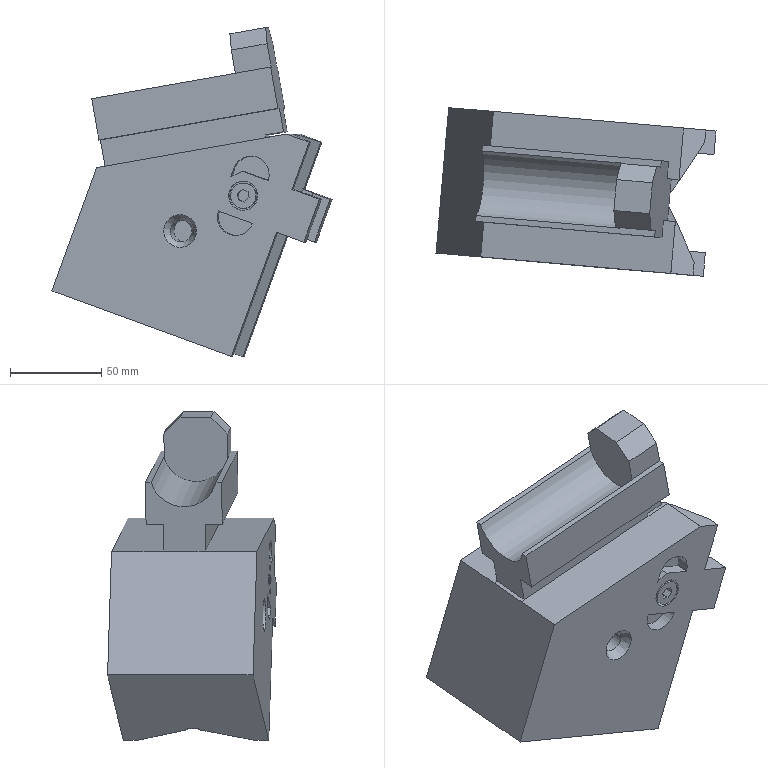Part | NX | features MAIN_BODY 2 | 1 solid | 106 faces | box 153.463 x 92.512 x 180.308 mm | volume 888038 mm3 | plane 93 | cylinder 9 | spline 2 | cone 2 | commonest cylinder face diameters 20 x4 12 x2 14 x2 37 x1